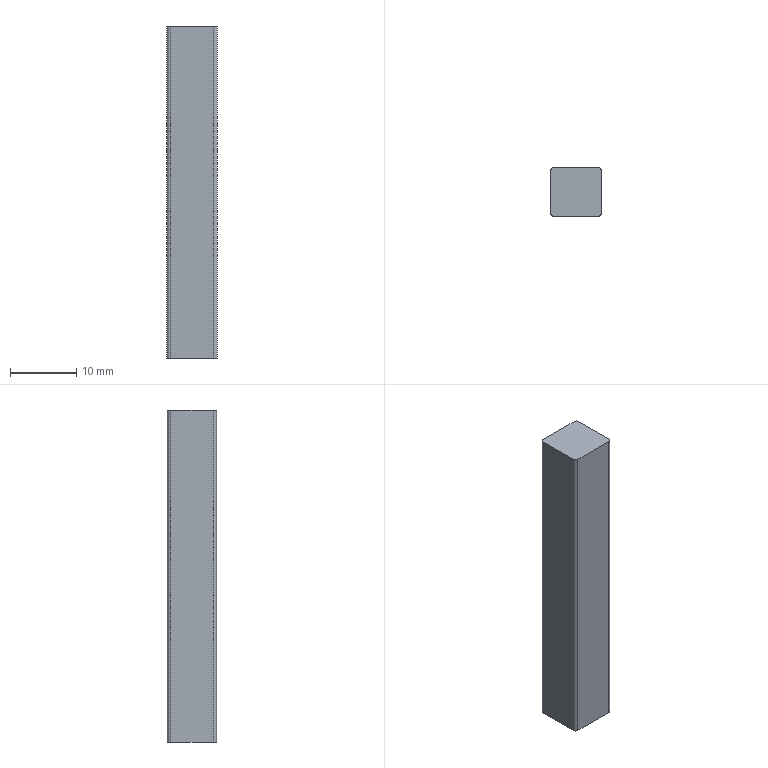Part | NX | features BREP 1 | 1 solid | 10 faces | box 7.6 x 7.4 x 50 mm | volume 2801 mm3 | plane 6 | cylinder 4 | commonest cylinder face diameters 1 x4
STEP:
#1=CARTESIAN_POINT('',(-3.3,3.7,-40.6));
#2=VERTEX_POINT('',#1);
#3=CARTESIAN_POINT('',(-3.8,3.2,-40.6));
#4=VERTEX_POINT('',#3);
#5=CARTESIAN_POINT('',(-3.3,3.2,-40.6));
#6=DIRECTION('',(0.,0.,1.));
#7=DIRECTION('',(1.,0.,0.));
#8=AXIS2_PLACEMENT_3D('',#5,#6,#7);
#9=CIRCLE('',#8,0.5);
#10=EDGE_CURVE('',#2,#4,#9,.T.);
#11=ORIENTED_EDGE('',*,*,#10,.F.);
#12=CARTESIAN_POINT('',(-3.3,3.7,-90.6));
#13=VERTEX_POINT('',#12);
#14=CARTESIAN_POINT('',(-3.3,3.7,-90.6));
#15=DIRECTION('',(0.,0.,1.));
#16=VECTOR('',#15,1000.);
#17=LINE('',#14,#16);
#18=EDGE_CURVE('',#13,#2,#17,.T.);
#19=ORIENTED_EDGE('',*,*,#18,.F.);
#20=CARTESIAN_POINT('',(-3.8,3.2,-90.6));
#21=VERTEX_POINT('',#20);
#22=CARTESIAN_POINT('',(-3.3,3.2,-90.6));
#23=DIRECTION('',(0.,0.,1.));
#24=DIRECTION('',(1.,0.,0.));
#25=AXIS2_PLACEMENT_3D('',#22,#23,#24);
#26=CIRCLE('',#25,0.5);
#27=EDGE_CURVE('',#13,#21,#26,.T.);
#28=ORIENTED_EDGE('',*,*,#27,.T.);
#29=CARTESIAN_POINT('',(-3.8,3.2,-90.6));
#30=DIRECTION('',(0.,0.,1.));
#31=VECTOR('',#30,1000.);
#32=LINE('',#29,#31);
#33=EDGE_CURVE('',#21,#4,#32,.T.);
#34=ORIENTED_EDGE('',*,*,#33,.T.);
#35=EDGE_LOOP('',(#11,#19,#28,#34));
#36=FACE_BOUND('',#35,.T.);
#37=CARTESIAN_POINT('',(-3.3,3.2,-90.6));
#38=DIRECTION('',(0.,0.,1.));
#39=DIRECTION('',(-1.,0.,0.));
#40=AXIS2_PLACEMENT_3D('',#37,#38,#39);
#41=CYLINDRICAL_SURFACE('',#40,0.5);
#42=ADVANCED_FACE('',(#36),#41,.T.);
#43=CARTESIAN_POINT('',(-3.8,-3.2,-40.6));
#44=VERTEX_POINT('',#43);
#45=CARTESIAN_POINT('',(-3.8,-3.2,-40.6));
#46=DIRECTION('',(0.,1.,0.));
#47=VECTOR('',#46,1000.);
#48=LINE('',#45,#47);
#49=EDGE_CURVE('',#44,#4,#48,.T.);
#50=ORIENTED_EDGE('',*,*,#49,.T.);
#51=ORIENTED_EDGE('',*,*,#33,.F.);
#52=CARTESIAN_POINT('',(-3.8,-3.2,-90.6));
#53=VERTEX_POINT('',#52);
#54=CARTESIAN_POINT('',(-3.8,-3.2,-90.6));
#55=DIRECTION('',(0.,1.,0.));
#56=VECTOR('',#55,1000.);
#57=LINE('',#54,#56);
#58=EDGE_CURVE('',#53,#21,#57,.T.);
#59=ORIENTED_EDGE('',*,*,#58,.F.);
#60=CARTESIAN_POINT('',(-3.8,-3.2,-90.6));
#61=DIRECTION('',(0.,0.,1.));
#62=VECTOR('',#61,1000.);
#63=LINE('',#60,#62);
#64=EDGE_CURVE('',#53,#44,#63,.T.);
#65=ORIENTED_EDGE('',*,*,#64,.T.);
#66=EDGE_LOOP('',(#50,#51,#59,#65));
#67=FACE_BOUND('',#66,.T.);
#68=CARTESIAN_POINT('',(-3.8,-3.2,-90.6));
#69=DIRECTION('',(1.,0.,0.));
#70=DIRECTION('',(0.,0.,1.));
#71=AXIS2_PLACEMENT_3D('',#68,#69,#70);
#72=PLANE('',#71);
#73=ADVANCED_FACE('',(#67),#72,.F.);
#74=CARTESIAN_POINT('',(-3.3,-3.7,-40.6));
#75=VERTEX_POINT('',#74);
#76=CARTESIAN_POINT('',(-3.3,-3.2,-40.6));
#77=DIRECTION('',(0.,0.,1.));
#78=DIRECTION('',(1.,0.,0.));
#79=AXIS2_PLACEMENT_3D('',#76,#77,#78);
#80=CIRCLE('',#79,0.5);
#81=EDGE_CURVE('',#44,#75,#80,.T.);
#82=ORIENTED_EDGE('',*,*,#81,.F.);
#83=ORIENTED_EDGE('',*,*,#64,.F.);
#84=CARTESIAN_POINT('',(-3.3,-3.7,-90.6));
#85=VERTEX_POINT('',#84);
#86=CARTESIAN_POINT('',(-3.3,-3.2,-90.6));
#87=DIRECTION('',(0.,0.,1.));
#88=DIRECTION('',(1.,0.,0.));
#89=AXIS2_PLACEMENT_3D('',#86,#87,#88);
#90=CIRCLE('',#89,0.5);
#91=EDGE_CURVE('',#53,#85,#90,.T.);
#92=ORIENTED_EDGE('',*,*,#91,.T.);
#93=CARTESIAN_POINT('',(-3.3,-3.7,-90.6));
#94=DIRECTION('',(0.,0.,1.));
#95=VECTOR('',#94,1000.);
#96=LINE('',#93,#95);
#97=EDGE_CURVE('',#85,#75,#96,.T.);
#98=ORIENTED_EDGE('',*,*,#97,.T.);
#99=EDGE_LOOP('',(#82,#83,#92,#98));
#100=FACE_BOUND('',#99,.T.);
#101=CARTESIAN_POINT('',(-3.3,-3.2,-90.6));
#102=DIRECTION('',(0.,0.,1.));
#103=DIRECTION('',(-1.,0.,0.));
#104=AXIS2_PLACEMENT_3D('',#101,#102,#103);
#105=CYLINDRICAL_SURFACE('',#104,0.5);
#106=ADVANCED_FACE('',(#100),#105,.T.);
#107=CARTESIAN_POINT('',(3.3,-3.7,-40.6));
#108=VERTEX_POINT('',#107);
#109=CARTESIAN_POINT('',(3.3,-3.7,-40.6));
#110=DIRECTION('',(-1.,0.,0.));
#111=VECTOR('',#110,1000.);
#112=LINE('',#109,#111);
#113=EDGE_CURVE('',#108,#75,#112,.T.);
#114=ORIENTED_EDGE('',*,*,#113,.T.);
#115=ORIENTED_EDGE('',*,*,#97,.F.);
#116=CARTESIAN_POINT('',(3.3,-3.7,-90.6));
#117=VERTEX_POINT('',#116);
#118=CARTESIAN_POINT('',(3.3,-3.7,-90.6));
#119=DIRECTION('',(-1.,0.,0.));
#120=VECTOR('',#119,1000.);
#121=LINE('',#118,#120);
#122=EDGE_CURVE('',#117,#85,#121,.T.);
#123=ORIENTED_EDGE('',*,*,#122,.F.);
#124=CARTESIAN_POINT('',(3.3,-3.7,-90.6));
#125=DIRECTION('',(0.,0.,1.));
#126=VECTOR('',#125,1000.);
#127=LINE('',#124,#126);
#128=EDGE_CURVE('',#117,#108,#127,.T.);
#129=ORIENTED_EDGE('',*,*,#128,.T.);
#130=EDGE_LOOP('',(#114,#115,#123,#129));
#131=FACE_BOUND('',#130,.T.);
#132=CARTESIAN_POINT('',(3.3,-3.7,-90.6));
#133=DIRECTION('',(0.,1.,0.));
#134=DIRECTION('',(0.,0.,-1.));
#135=AXIS2_PLACEMENT_3D('',#132,#133,#134);
#136=PLANE('',#135);
#137=ADVANCED_FACE('',(#131),#136,.F.);
#138=CARTESIAN_POINT('',(3.8,-3.2,-40.6));
#139=VERTEX_POINT('',#138);
#140=CARTESIAN_POINT('',(3.3,-3.2,-40.6));
#141=DIRECTION('',(0.,0.,1.));
#142=DIRECTION('',(1.,0.,0.));
#143=AXIS2_PLACEMENT_3D('',#140,#141,#142);
#144=CIRCLE('',#143,0.5);
#145=EDGE_CURVE('',#108,#139,#144,.T.);
#146=ORIENTED_EDGE('',*,*,#145,.F.);
#147=ORIENTED_EDGE('',*,*,#128,.F.);
#148=CARTESIAN_POINT('',(3.8,-3.2,-90.6));
#149=VERTEX_POINT('',#148);
#150=CARTESIAN_POINT('',(3.3,-3.2,-90.6));
#151=DIRECTION('',(0.,0.,1.));
#152=DIRECTION('',(1.,0.,0.));
#153=AXIS2_PLACEMENT_3D('',#150,#151,#152);
#154=CIRCLE('',#153,0.5);
#155=EDGE_CURVE('',#117,#149,#154,.T.);
#156=ORIENTED_EDGE('',*,*,#155,.T.);
#157=CARTESIAN_POINT('',(3.8,-3.2,-90.6));
#158=DIRECTION('',(0.,0.,1.));
#159=VECTOR('',#158,1000.);
#160=LINE('',#157,#159);
#161=EDGE_CURVE('',#149,#139,#160,.T.);
#162=ORIENTED_EDGE('',*,*,#161,.T.);
#163=EDGE_LOOP('',(#146,#147,#156,#162));
#164=FACE_BOUND('',#163,.T.);
#165=CARTESIAN_POINT('',(3.3,-3.2,-90.6));
#166=DIRECTION('',(0.,0.,1.));
#167=DIRECTION('',(-1.,0.,0.));
#168=AXIS2_PLACEMENT_3D('',#165,#166,#167);
#169=CYLINDRICAL_SURFACE('',#168,0.5);
#170=ADVANCED_FACE('',(#164),#169,.T.);
#171=CARTESIAN_POINT('',(3.8,3.2,-40.6));
#172=VERTEX_POINT('',#171);
#173=CARTESIAN_POINT('',(3.8,3.2,-40.6));
#174=DIRECTION('',(0.,-1.,0.));
#175=VECTOR('',#174,1000.);
#176=LINE('',#173,#175);
#177=EDGE_CURVE('',#172,#139,#176,.T.);
#178=ORIENTED_EDGE('',*,*,#177,.T.);
#179=ORIENTED_EDGE('',*,*,#161,.F.);
#180=CARTESIAN_POINT('',(3.8,3.2,-90.6));
#181=VERTEX_POINT('',#180);
#182=CARTESIAN_POINT('',(3.8,3.2,-90.6));
#183=DIRECTION('',(0.,-1.,0.));
#184=VECTOR('',#183,1000.);
#185=LINE('',#182,#184);
#186=EDGE_CURVE('',#181,#149,#185,.T.);
#187=ORIENTED_EDGE('',*,*,#186,.F.);
#188=CARTESIAN_POINT('',(3.8,3.2,-90.6));
#189=DIRECTION('',(0.,0.,1.));
#190=VECTOR('',#189,1000.);
#191=LINE('',#188,#190);
#192=EDGE_CURVE('',#181,#172,#191,.T.);
#193=ORIENTED_EDGE('',*,*,#192,.T.);
#194=EDGE_LOOP('',(#178,#179,#187,#193));
#195=FACE_BOUND('',#194,.T.);
#196=CARTESIAN_POINT('',(3.8,3.2,-90.6));
#197=DIRECTION('',(-1.,0.,0.));
#198=DIRECTION('',(0.,0.,-1.));
#199=AXIS2_PLACEMENT_3D('',#196,#197,#198);
#200=PLANE('',#199);
#201=ADVANCED_FACE('',(#195),#200,.F.);
#202=CARTESIAN_POINT('',(3.3,3.7,-40.6));
#203=VERTEX_POINT('',#202);
#204=CARTESIAN_POINT('',(3.3,3.2,-40.6));
#205=DIRECTION('',(0.,0.,1.));
#206=DIRECTION('',(1.,0.,0.));
#207=AXIS2_PLACEMENT_3D('',#204,#205,#206);
#208=CIRCLE('',#207,0.5);
#209=EDGE_CURVE('',#172,#203,#208,.T.);
#210=ORIENTED_EDGE('',*,*,#209,.F.);
#211=ORIENTED_EDGE('',*,*,#192,.F.);
#212=CARTESIAN_POINT('',(3.3,3.7,-90.6));
#213=VERTEX_POINT('',#212);
#214=CARTESIAN_POINT('',(3.3,3.2,-90.6));
#215=DIRECTION('',(0.,0.,1.));
#216=DIRECTION('',(1.,0.,0.));
#217=AXIS2_PLACEMENT_3D('',#214,#215,#216);
#218=CIRCLE('',#217,0.5);
#219=EDGE_CURVE('',#181,#213,#218,.T.);
#220=ORIENTED_EDGE('',*,*,#219,.T.);
#221=CARTESIAN_POINT('',(3.3,3.7,-90.6));
#222=DIRECTION('',(0.,0.,1.));
#223=VECTOR('',#222,1000.);
#224=LINE('',#221,#223);
#225=EDGE_CURVE('',#213,#203,#224,.T.);
#226=ORIENTED_EDGE('',*,*,#225,.T.);
#227=EDGE_LOOP('',(#210,#211,#220,#226));
#228=FACE_BOUND('',#227,.T.);
#229=CARTESIAN_POINT('',(3.3,3.2,-90.6));
#230=DIRECTION('',(0.,0.,1.));
#231=DIRECTION('',(-1.,0.,0.));
#232=AXIS2_PLACEMENT_3D('',#229,#230,#231);
#233=CYLINDRICAL_SURFACE('',#232,0.5);
#234=ADVANCED_FACE('',(#228),#233,.T.);
#235=CARTESIAN_POINT('',(-3.3,3.7,-40.6));
#236=DIRECTION('',(1.,0.,0.));
#237=VECTOR('',#236,1000.);
#238=LINE('',#235,#237);
#239=EDGE_CURVE('',#2,#203,#238,.T.);
#240=ORIENTED_EDGE('',*,*,#239,.T.);
#241=ORIENTED_EDGE('',*,*,#225,.F.);
#242=CARTESIAN_POINT('',(-3.3,3.7,-90.6));
#243=DIRECTION('',(1.,0.,0.));
#244=VECTOR('',#243,1000.);
#245=LINE('',#242,#244);
#246=EDGE_CURVE('',#13,#213,#245,.T.);
#247=ORIENTED_EDGE('',*,*,#246,.F.);
#248=ORIENTED_EDGE('',*,*,#18,.T.);
#249=EDGE_LOOP('',(#240,#241,#247,#248));
#250=FACE_BOUND('',#249,.T.);
#251=CARTESIAN_POINT('',(-3.3,3.7,-90.6));
#252=DIRECTION('',(0.,-1.,0.));
#253=DIRECTION('',(0.,0.,1.));
#254=AXIS2_PLACEMENT_3D('',#251,#252,#253);
#255=PLANE('',#254);
#256=ADVANCED_FACE('',(#250),#255,.F.);
#257=ORIENTED_EDGE('',*,*,#27,.F.);
#258=ORIENTED_EDGE('',*,*,#246,.T.);
#259=ORIENTED_EDGE('',*,*,#219,.F.);
#260=ORIENTED_EDGE('',*,*,#186,.T.);
#261=ORIENTED_EDGE('',*,*,#155,.F.);
#262=ORIENTED_EDGE('',*,*,#122,.T.);
#263=ORIENTED_EDGE('',*,*,#91,.F.);
#264=ORIENTED_EDGE('',*,*,#58,.T.);
#265=EDGE_LOOP('',(#257,#258,#259,#260,#261,#262,#263,#264));
#266=FACE_BOUND('',#265,.T.);
#267=CARTESIAN_POINT('',(-3.3,3.2,-90.6));
#268=DIRECTION('',(0.,0.,1.));
#269=DIRECTION('',(-1.,0.,0.));
#270=AXIS2_PLACEMENT_3D('',#267,#268,#269);
#271=PLANE('',#270);
#272=ADVANCED_FACE('',(#266),#271,.F.);
#273=ORIENTED_EDGE('',*,*,#10,.T.);
#274=ORIENTED_EDGE('',*,*,#49,.F.);
#275=ORIENTED_EDGE('',*,*,#81,.T.);
#276=ORIENTED_EDGE('',*,*,#113,.F.);
#277=ORIENTED_EDGE('',*,*,#145,.T.);
#278=ORIENTED_EDGE('',*,*,#177,.F.);
#279=ORIENTED_EDGE('',*,*,#209,.T.);
#280=ORIENTED_EDGE('',*,*,#239,.F.);
#281=EDGE_LOOP('',(#273,#274,#275,#276,#277,#278,#279,#280));
#282=FACE_BOUND('',#281,.T.);
#283=CARTESIAN_POINT('',(-3.3,3.2,-40.6));
#284=DIRECTION('',(0.,0.,1.));
#285=DIRECTION('',(-1.,0.,0.));
#286=AXIS2_PLACEMENT_3D('',#283,#284,#285);
#287=PLANE('',#286);
#288=ADVANCED_FACE('',(#282),#287,.T.);
#289=CLOSED_SHELL('',(#42,#73,#106,#137,#170,#201,#234,#256,#272,#288));
#290=MANIFOLD_SOLID_BREP('',#289);
#291=(LENGTH_UNIT()NAMED_UNIT(*)SI_UNIT(.MILLI.,.METRE.));
#292=UNCERTAINTY_MEASURE_WITH_UNIT(LENGTH_MEASURE(0.00001),#291,'','');
#293=(NAMED_UNIT(*)PLANE_ANGLE_UNIT()SI_UNIT($,.RADIAN.));
#294=(NAMED_UNIT(*)SI_UNIT($,.STERADIAN.)SOLID_ANGLE_UNIT());
#295=(GEOMETRIC_REPRESENTATION_CONTEXT(3)GLOBAL_UNCERTAINTY_ASSIGNED_CONTEXT((#292))GLOBAL_UNIT_ASSIGNED_CONTEXT((#291,#293,#294))REPRESENTATION_CONTEXT('',''));
#296=ADVANCED_BREP_SHAPE_REPRESENTATION('',(#290),#295);